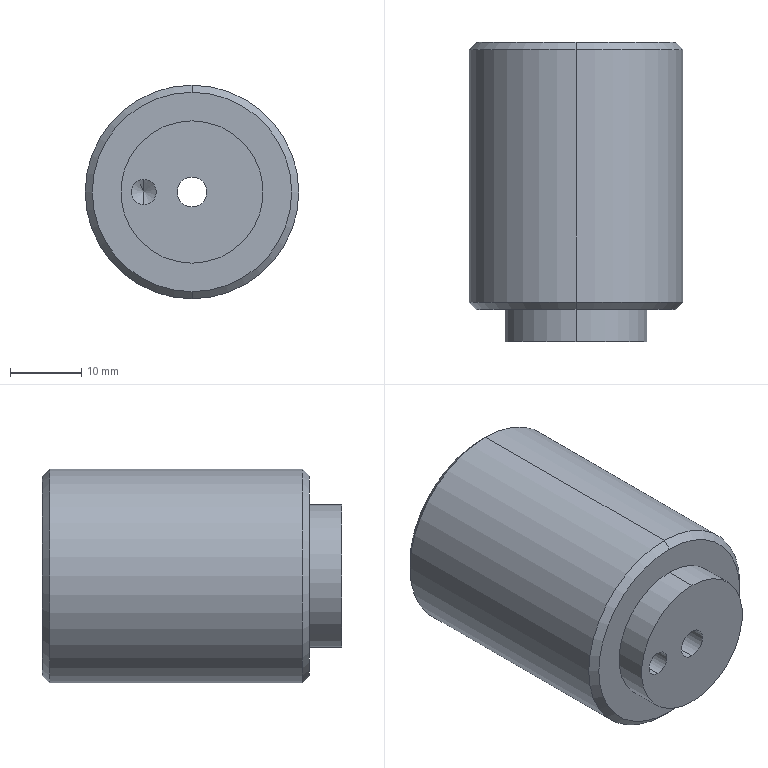Part | STEP file | Rotating shaft | 1 solid | 25 faces | box 30 x 42 x 30 mm | volume 17511 mm3 | cylinder 10 | cone 8 | plane 7 | commonest cylinder face diameters 3.5 x2 4.2 x2 19 x2 20 x2 30 x2